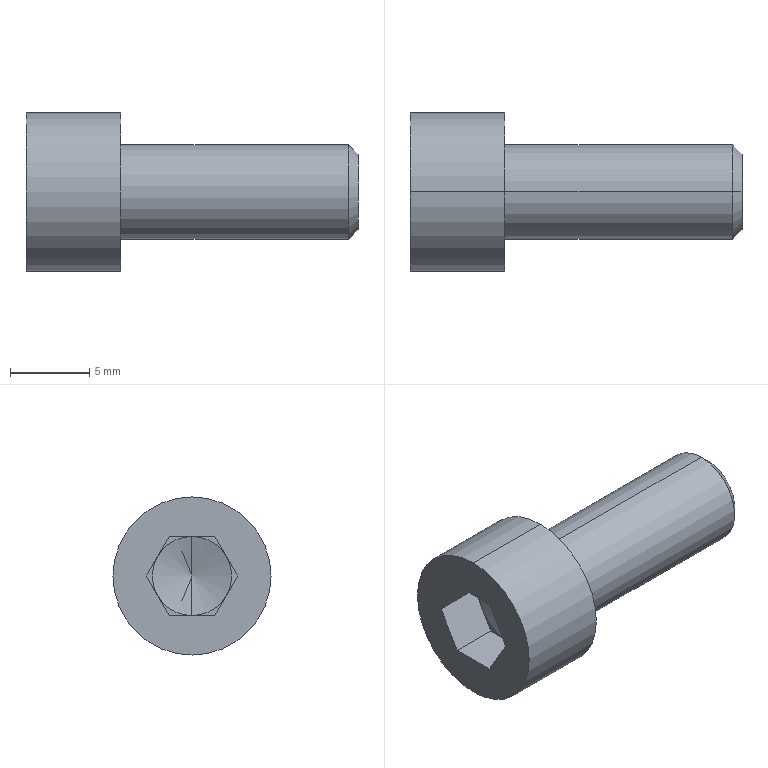Part | STEP file | 0232_301_CBM6-15 | 1 solid | 23 faces | box 21 x 10 x 10 mm | volume 822.712 mm3 | plane 15 | cylinder 4 | cone 4 | commonest cylinder face diameters 6 x2 10 x2
STEP:
#1=CARTESIAN_POINT('',(0.,0.,0.));
#2=DIRECTION('',(0.,0.,1.));
#3=DIRECTION('',(1.,0.,0.));
#4=AXIS2_PLACEMENT_3D('',#1,#2,#3);
#5=CARTESIAN_POINT('',(0.,0.,-3.));
#6=VERTEX_POINT('',#5);
#7=CARTESIAN_POINT('',(0.,0.,3.));
#8=VERTEX_POINT('',#7);
#9=CARTESIAN_POINT('',(0.,0.,0.));
#10=DIRECTION('',(1.,0.,0.));
#11=DIRECTION('',(0.,0.,-1.));
#12=AXIS2_PLACEMENT_3D('',#9,#10,#11);
#13=CIRCLE('',#12,3.);
#14=CARTESIAN_POINT('',(7.193,0.,0.));
#15=DIRECTION('',(1.,0.,0.));
#16=DIRECTION('',(0.,0.,-1.));
#17=AXIS2_PLACEMENT_3D('',#14,#15,#16);
#18=CYLINDRICAL_SURFACE('',#17,3.);
#19=CARTESIAN_POINT('',(0.,-7.193));
#20=DIRECTION('',(1.,0.));
#21=VECTOR('',#20,1.);
#22=LINE('',#19,#21);
#23=(GEOMETRIC_REPRESENTATION_CONTEXT(2)PARAMETRIC_REPRESENTATION_CONTEXT()REPRESENTATION_CONTEXT('',''));
#24=DEFINITIONAL_REPRESENTATION('',(#22),#23);
#25=PCURVE('',#18,#24);
#26=CARTESIAN_POINT('',(0.,4.,0.));
#27=DIRECTION('',(1.,0.,0.));
#28=DIRECTION('',(0.,0.,-1.));
#29=AXIS2_PLACEMENT_3D('',#26,#27,#28);
#30=PLANE('',#29);
#31=CARTESIAN_POINT('',(0.,-4.));
#32=DIRECTION('',(1.,0.));
#33=AXIS2_PLACEMENT_2D('',#31,#32);
#34=CIRCLE('',#33,3.);
#35=(GEOMETRIC_REPRESENTATION_CONTEXT(2)PARAMETRIC_REPRESENTATION_CONTEXT()REPRESENTATION_CONTEXT('',''));
#36=DEFINITIONAL_REPRESENTATION('',(#34),#35);
#37=PCURVE('',#30,#36);
#38=SURFACE_CURVE('',#13,(#25,#37),.PCURVE_S1.);
#39=EDGE_CURVE('',#6,#8,#38,.T.);
#40=ORIENTED_EDGE('',*,*,#39,.T.);
#41=CARTESIAN_POINT('',(14.386,0.,3.));
#42=VERTEX_POINT('',#41);
#43=CARTESIAN_POINT('',(7.193,0.,3.));
#44=DIRECTION('',(1.,0.,0.));
#45=VECTOR('',#44,1.);
#46=LINE('',#43,#45);
#47=CARTESIAN_POINT('',(3.142,0.));
#48=DIRECTION('',(0.,1.));
#49=VECTOR('',#48,1.);
#50=LINE('',#47,#49);
#51=(GEOMETRIC_REPRESENTATION_CONTEXT(2)PARAMETRIC_REPRESENTATION_CONTEXT()REPRESENTATION_CONTEXT('',''));
#52=DEFINITIONAL_REPRESENTATION('',(#50),#51);
#53=PCURVE('',#18,#52);
#54=CARTESIAN_POINT('',(7.193,0.,0.));
#55=DIRECTION('',(1.,0.,0.));
#56=DIRECTION('',(0.,0.,-1.));
#57=AXIS2_PLACEMENT_3D('',#54,#55,#56);
#58=CYLINDRICAL_SURFACE('',#57,3.);
#59=CARTESIAN_POINT('',(3.142,0.));
#60=DIRECTION('',(0.,1.));
#61=VECTOR('',#60,1.);
#62=LINE('',#59,#61);
#63=(GEOMETRIC_REPRESENTATION_CONTEXT(2)PARAMETRIC_REPRESENTATION_CONTEXT()REPRESENTATION_CONTEXT('',''));
#64=DEFINITIONAL_REPRESENTATION('',(#62),#63);
#65=PCURVE('',#58,#64);
#66=SURFACE_CURVE('',#46,(#53,#65),.PCURVE_S1.);
#67=EDGE_CURVE('',#8,#42,#66,.T.);
#68=ORIENTED_EDGE('',*,*,#67,.T.);
#69=CARTESIAN_POINT('',(14.386,0.,-3.));
#70=VERTEX_POINT('',#69);
#71=CARTESIAN_POINT('',(14.386,0.,0.));
#72=DIRECTION('',(-1.,0.,0.));
#73=DIRECTION('',(0.,0.,-1.));
#74=AXIS2_PLACEMENT_3D('',#71,#72,#73);
#75=CIRCLE('',#74,3.);
#76=CARTESIAN_POINT('',(6.283,7.193));
#77=DIRECTION('',(-1.,0.));
#78=VECTOR('',#77,1.);
#79=LINE('',#76,#78);
#80=(GEOMETRIC_REPRESENTATION_CONTEXT(2)PARAMETRIC_REPRESENTATION_CONTEXT()REPRESENTATION_CONTEXT('',''));
#81=DEFINITIONAL_REPRESENTATION('',(#79),#80);
#82=PCURVE('',#18,#81);
#83=CARTESIAN_POINT('',(14.387,0.,0.));
#84=DIRECTION('',(-1.,0.,0.));
#85=DIRECTION('',(0.,0.,1.));
#86=AXIS2_PLACEMENT_3D('',#83,#84,#85);
#87=CONICAL_SURFACE('',#86,3.,0.7854);
#88=CARTESIAN_POINT('',(-3.142,0.));
#89=DIRECTION('',(1.,0.));
#90=VECTOR('',#89,1.);
#91=LINE('',#88,#90);
#92=(GEOMETRIC_REPRESENTATION_CONTEXT(2)PARAMETRIC_REPRESENTATION_CONTEXT()REPRESENTATION_CONTEXT('',''));
#93=DEFINITIONAL_REPRESENTATION('',(#91),#92);
#94=PCURVE('',#87,#93);
#95=SURFACE_CURVE('',#75,(#82,#94),.PCURVE_S1.);
#96=EDGE_CURVE('',#42,#70,#95,.T.);
#97=ORIENTED_EDGE('',*,*,#96,.T.);
#98=CARTESIAN_POINT('',(7.193,0.,-3.));
#99=DIRECTION('',(1.,0.,0.));
#100=VECTOR('',#99,1.);
#101=LINE('',#98,#100);
#102=CARTESIAN_POINT('',(0.,0.));
#103=DIRECTION('',(0.,1.));
#104=VECTOR('',#103,1.);
#105=LINE('',#102,#104);
#106=(GEOMETRIC_REPRESENTATION_CONTEXT(2)PARAMETRIC_REPRESENTATION_CONTEXT()REPRESENTATION_CONTEXT('',''));
#107=DEFINITIONAL_REPRESENTATION('',(#105),#106);
#108=PCURVE('',#18,#107);
#109=CARTESIAN_POINT('',(6.283,0.));
#110=DIRECTION('',(0.,1.));
#111=VECTOR('',#110,1.);
#112=LINE('',#109,#111);
#113=(GEOMETRIC_REPRESENTATION_CONTEXT(2)PARAMETRIC_REPRESENTATION_CONTEXT()REPRESENTATION_CONTEXT('',''));
#114=DEFINITIONAL_REPRESENTATION('',(#112),#113);
#115=PCURVE('',#58,#114);
#116=SURFACE_CURVE('',#101,(#108,#115),.PCURVE_S1.);
#117=EDGE_CURVE('',#6,#70,#116,.T.);
#118=ORIENTED_EDGE('',*,*,#117,.F.);
#119=EDGE_LOOP('',(#40,#68,#97,#118));
#120=FACE_BOUND('',#119,.T.);
#121=ADVANCED_FACE('',(#120),#18,.T.);
#122=CARTESIAN_POINT('',(15.,0.,2.386));
#123=VERTEX_POINT('',#122);
#124=CARTESIAN_POINT('',(15.,0.,-2.386));
#125=VERTEX_POINT('',#124);
#126=CARTESIAN_POINT('',(15.,0.,0.));
#127=DIRECTION('',(-1.,0.,0.));
#128=DIRECTION('',(0.,0.,1.));
#129=AXIS2_PLACEMENT_3D('',#126,#127,#128);
#130=CIRCLE('',#129,2.386);
#131=CARTESIAN_POINT('',(0.,-0.6135));
#132=DIRECTION('',(1.,0.));
#133=VECTOR('',#132,1.);
#134=LINE('',#131,#133);
#135=(GEOMETRIC_REPRESENTATION_CONTEXT(2)PARAMETRIC_REPRESENTATION_CONTEXT()REPRESENTATION_CONTEXT('',''));
#136=DEFINITIONAL_REPRESENTATION('',(#134),#135);
#137=PCURVE('',#87,#136);
#138=CARTESIAN_POINT('',(15.,1.193,0.));
#139=DIRECTION('',(1.,0.,0.));
#140=DIRECTION('',(0.,0.,-1.));
#141=AXIS2_PLACEMENT_3D('',#138,#139,#140);
#142=PLANE('',#141);
#143=CARTESIAN_POINT('',(-2.386,-1.193));
#144=CARTESIAN_POINT('',(-2.386,2.94));
#145=CARTESIAN_POINT('',(1.193,0.8735));
#146=CARTESIAN_POINT('',(4.773,-1.193));
#147=CARTESIAN_POINT('',(1.193,-3.26));
#148=CARTESIAN_POINT('',(-2.386,-5.327));
#149=CARTESIAN_POINT('',(-2.386,-1.193));
#150=(BOUNDED_CURVE()B_SPLINE_CURVE(2,(#143,#144,#145,#146,#147,#148,#149),.UNSPECIFIED.,.T.,.F.)B_SPLINE_CURVE_WITH_KNOTS((1,2,2,2,2,1),(-2.094,0.,2.094,4.189,6.283,8.378),.UNSPECIFIED.)CURVE()GEOMETRIC_REPRESENTATION_ITEM()RATIONAL_B_SPLINE_CURVE((1.,0.5,1.,0.5,1.,0.5,1.))REPRESENTATION_ITEM(''));
#151=(GEOMETRIC_REPRESENTATION_CONTEXT(2)PARAMETRIC_REPRESENTATION_CONTEXT()REPRESENTATION_CONTEXT('',''));
#152=DEFINITIONAL_REPRESENTATION('',(#150),#151);
#153=PCURVE('',#142,#152);
#154=SURFACE_CURVE('',#130,(#137,#153),.PCURVE_S1.);
#155=EDGE_CURVE('',#123,#125,#154,.T.);
#156=ORIENTED_EDGE('',*,*,#155,.T.);
#157=CARTESIAN_POINT('',(14.387,0.,-3.));
#158=DIRECTION('',(-0.7071,0.,-0.7071));
#159=VECTOR('',#158,1.);
#160=LINE('',#157,#159);
#161=CARTESIAN_POINT('',(3.142,0.));
#162=DIRECTION('',(0.,1.));
#163=VECTOR('',#162,1.);
#164=LINE('',#161,#163);
#165=(GEOMETRIC_REPRESENTATION_CONTEXT(2)PARAMETRIC_REPRESENTATION_CONTEXT()REPRESENTATION_CONTEXT('',''));
#166=DEFINITIONAL_REPRESENTATION('',(#164),#165);
#167=PCURVE('',#87,#166);
#168=CARTESIAN_POINT('',(14.387,0.,0.));
#169=DIRECTION('',(-1.,0.,0.));
#170=DIRECTION('',(0.,0.,1.));
#171=AXIS2_PLACEMENT_3D('',#168,#169,#170);
#172=CONICAL_SURFACE('',#171,3.,0.7854);
#173=CARTESIAN_POINT('',(3.142,0.));
#174=DIRECTION('',(0.,1.));
#175=VECTOR('',#174,1.);
#176=LINE('',#173,#175);
#177=(GEOMETRIC_REPRESENTATION_CONTEXT(2)PARAMETRIC_REPRESENTATION_CONTEXT()REPRESENTATION_CONTEXT('',''));
#178=DEFINITIONAL_REPRESENTATION('',(#176),#177);
#179=PCURVE('',#172,#178);
#180=SURFACE_CURVE('',#160,(#167,#179),.PCURVE_S1.);
#181=EDGE_CURVE('',#125,#70,#180,.T.);
#182=ORIENTED_EDGE('',*,*,#181,.T.);
#183=ORIENTED_EDGE('',*,*,#96,.F.);
#184=CARTESIAN_POINT('',(14.387,0.,3.));
#185=DIRECTION('',(-0.7071,0.,0.7071));
#186=VECTOR('',#185,1.);
#187=LINE('',#184,#186);
#188=CARTESIAN_POINT('',(0.,0.));
#189=DIRECTION('',(0.,1.));
#190=VECTOR('',#189,1.);
#191=LINE('',#188,#190);
#192=(GEOMETRIC_REPRESENTATION_CONTEXT(2)PARAMETRIC_REPRESENTATION_CONTEXT()REPRESENTATION_CONTEXT('',''));
#193=DEFINITIONAL_REPRESENTATION('',(#191),#192);
#194=PCURVE('',#87,#193);
#195=CARTESIAN_POINT('',(6.283,0.));
#196=DIRECTION('',(0.,1.));
#197=VECTOR('',#196,1.);
#198=LINE('',#195,#197);
#199=(GEOMETRIC_REPRESENTATION_CONTEXT(2)PARAMETRIC_REPRESENTATION_CONTEXT()REPRESENTATION_CONTEXT('',''));
#200=DEFINITIONAL_REPRESENTATION('',(#198),#199);
#201=PCURVE('',#172,#200);
#202=SURFACE_CURVE('',#187,(#194,#201),.PCURVE_S1.);
#203=EDGE_CURVE('',#123,#42,#202,.T.);
#204=ORIENTED_EDGE('',*,*,#203,.F.);
#205=EDGE_LOOP('',(#156,#182,#183,#204));
#206=FACE_BOUND('',#205,.T.);
#207=ADVANCED_FACE('',(#206),#87,.T.);
#208=CARTESIAN_POINT('',(-6.,0.,-5.));
#209=VERTEX_POINT('',#208);
#210=CARTESIAN_POINT('',(-6.,0.,5.));
#211=VERTEX_POINT('',#210);
#212=CARTESIAN_POINT('',(-6.,0.,0.));
#213=DIRECTION('',(1.,0.,0.));
#214=DIRECTION('',(0.,0.,-1.));
#215=AXIS2_PLACEMENT_3D('',#212,#213,#214);
#216=CIRCLE('',#215,5.);
#217=CARTESIAN_POINT('',(-3.,0.,0.));
#218=DIRECTION('',(1.,0.,0.));
#219=DIRECTION('',(0.,0.,-1.));
#220=AXIS2_PLACEMENT_3D('',#217,#218,#219);
#221=CYLINDRICAL_SURFACE('',#220,5.);
#222=CARTESIAN_POINT('',(0.,-3.));
#223=DIRECTION('',(1.,0.));
#224=VECTOR('',#223,1.);
#225=LINE('',#222,#224);
#226=(GEOMETRIC_REPRESENTATION_CONTEXT(2)PARAMETRIC_REPRESENTATION_CONTEXT()REPRESENTATION_CONTEXT('',''));
#227=DEFINITIONAL_REPRESENTATION('',(#225),#226);
#228=PCURVE('',#221,#227);
#229=CARTESIAN_POINT('',(-6.,2.5,0.));
#230=DIRECTION('',(-1.,0.,0.));
#231=DIRECTION('',(0.,0.,1.));
#232=AXIS2_PLACEMENT_3D('',#229,#230,#231);
#233=PLANE('',#232);
#234=CARTESIAN_POINT('',(-5.,-2.5));
#235=CARTESIAN_POINT('',(-5.,6.16));
#236=CARTESIAN_POINT('',(2.5,1.83));
#237=CARTESIAN_POINT('',(10.,-2.5));
#238=CARTESIAN_POINT('',(2.5,-6.83));
#239=CARTESIAN_POINT('',(-5.,-11.16));
#240=CARTESIAN_POINT('',(-5.,-2.5));
#241=(BOUNDED_CURVE()B_SPLINE_CURVE(2,(#234,#235,#236,#237,#238,#239,#240),.UNSPECIFIED.,.T.,.F.)B_SPLINE_CURVE_WITH_KNOTS((1,2,2,2,2,1),(-2.094,0.,2.094,4.189,6.283,8.378),.UNSPECIFIED.)CURVE()GEOMETRIC_REPRESENTATION_ITEM()RATIONAL_B_SPLINE_CURVE((1.,0.5,1.,0.5,1.,0.5,1.))REPRESENTATION_ITEM(''));
#242=(GEOMETRIC_REPRESENTATION_CONTEXT(2)PARAMETRIC_REPRESENTATION_CONTEXT()REPRESENTATION_CONTEXT('',''));
#243=DEFINITIONAL_REPRESENTATION('',(#241),#242);
#244=PCURVE('',#233,#243);
#245=SURFACE_CURVE('',#216,(#228,#244),.PCURVE_S1.);
#246=EDGE_CURVE('',#209,#211,#245,.T.);
#247=ORIENTED_EDGE('',*,*,#246,.T.);
#248=CARTESIAN_POINT('',(0.,0.,5.));
#249=VERTEX_POINT('',#248);
#250=CARTESIAN_POINT('',(-3.,0.,5.));
#251=DIRECTION('',(1.,0.,0.));
#252=VECTOR('',#251,1.);
#253=LINE('',#250,#252);
#254=CARTESIAN_POINT('',(3.142,0.));
#255=DIRECTION('',(0.,1.));
#256=VECTOR('',#255,1.);
#257=LINE('',#254,#256);
#258=(GEOMETRIC_REPRESENTATION_CONTEXT(2)PARAMETRIC_REPRESENTATION_CONTEXT()REPRESENTATION_CONTEXT('',''));
#259=DEFINITIONAL_REPRESENTATION('',(#257),#258);
#260=PCURVE('',#221,#259);
#261=CARTESIAN_POINT('',(-3.,0.,0.));
#262=DIRECTION('',(1.,0.,0.));
#263=DIRECTION('',(0.,0.,-1.));
#264=AXIS2_PLACEMENT_3D('',#261,#262,#263);
#265=CYLINDRICAL_SURFACE('',#264,5.);
#266=CARTESIAN_POINT('',(3.142,0.));
#267=DIRECTION('',(0.,1.));
#268=VECTOR('',#267,1.);
#269=LINE('',#266,#268);
#270=(GEOMETRIC_REPRESENTATION_CONTEXT(2)PARAMETRIC_REPRESENTATION_CONTEXT()REPRESENTATION_CONTEXT('',''));
#271=DEFINITIONAL_REPRESENTATION('',(#269),#270);
#272=PCURVE('',#265,#271);
#273=SURFACE_CURVE('',#253,(#260,#272),.PCURVE_S1.);
#274=EDGE_CURVE('',#211,#249,#273,.T.);
#275=ORIENTED_EDGE('',*,*,#274,.T.);
#276=CARTESIAN_POINT('',(0.,0.,-5.));
#277=VERTEX_POINT('',#276);
#278=CARTESIAN_POINT('',(0.,0.,0.));
#279=DIRECTION('',(1.,0.,0.));
#280=DIRECTION('',(0.,0.,-1.));
#281=AXIS2_PLACEMENT_3D('',#278,#279,#280);
#282=CIRCLE('',#281,5.);
#283=CARTESIAN_POINT('',(0.,3.));
#284=DIRECTION('',(1.,0.));
#285=VECTOR('',#284,1.);
#286=LINE('',#283,#285);
#287=(GEOMETRIC_REPRESENTATION_CONTEXT(2)PARAMETRIC_REPRESENTATION_CONTEXT()REPRESENTATION_CONTEXT('',''));
#288=DEFINITIONAL_REPRESENTATION('',(#286),#287);
#289=PCURVE('',#221,#288);
#290=CARTESIAN_POINT('',(0.,-4.));
#291=DIRECTION('',(1.,0.));
#292=AXIS2_PLACEMENT_2D('',#290,#291);
#293=CIRCLE('',#292,5.);
#294=(GEOMETRIC_REPRESENTATION_CONTEXT(2)PARAMETRIC_REPRESENTATION_CONTEXT()REPRESENTATION_CONTEXT('',''));
#295=DEFINITIONAL_REPRESENTATION('',(#293),#294);
#296=PCURVE('',#30,#295);
#297=SURFACE_CURVE('',#282,(#289,#296),.PCURVE_S1.);
#298=EDGE_CURVE('',#277,#249,#297,.T.);
#299=ORIENTED_EDGE('',*,*,#298,.F.);
#300=CARTESIAN_POINT('',(-3.,0.,-5.));
#301=DIRECTION('',(1.,0.,0.));
#302=VECTOR('',#301,1.);
#303=LINE('',#300,#302);
#304=CARTESIAN_POINT('',(0.,0.));
#305=DIRECTION('',(0.,1.));
#306=VECTOR('',#305,1.);
#307=LINE('',#304,#306);
#308=(GEOMETRIC_REPRESENTATION_CONTEXT(2)PARAMETRIC_REPRESENTATION_CONTEXT()REPRESENTATION_CONTEXT('',''));
#309=DEFINITIONAL_REPRESENTATION('',(#307),#308);
#310=PCURVE('',#221,#309);
#311=CARTESIAN_POINT('',(6.283,0.));
#312=DIRECTION('',(0.,1.));
#313=VECTOR('',#312,1.);
#314=LINE('',#311,#313);
#315=(GEOMETRIC_REPRESENTATION_CONTEXT(2)PARAMETRIC_REPRESENTATION_CONTEXT()REPRESENTATION_CONTEXT('',''));
#316=DEFINITIONAL_REPRESENTATION('',(#314),#315);
#317=PCURVE('',#265,#316);
#318=SURFACE_CURVE('',#303,(#310,#317),.PCURVE_S1.);
#319=EDGE_CURVE('',#209,#277,#318,.T.);
#320=ORIENTED_EDGE('',*,*,#319,.F.);
#321=EDGE_LOOP('',(#247,#275,#299,#320));
#322=FACE_BOUND('',#321,.T.);
#323=ADVANCED_FACE('',(#322),#221,.T.);
#324=CARTESIAN_POINT('',(-3.,-2.165,1.25));
#325=VERTEX_POINT('',#324);
#326=CARTESIAN_POINT('',(-3.,0.,2.5));
#327=VERTEX_POINT('',#326);
#328=CARTESIAN_POINT('',(-3.,0.,0.));
#329=DIRECTION('',(-1.,0.,0.));
#330=DIRECTION('',(0.,0.,1.));
#331=AXIS2_PLACEMENT_3D('',#328,#329,#330);
#332=CIRCLE('',#331,2.5);
#333=CARTESIAN_POINT('',(-3.,0.,0.));
#334=DIRECTION('',(-1.,0.,0.));
#335=DIRECTION('',(0.,0.,1.));
#336=AXIS2_PLACEMENT_3D('',#333,#334,#335);
#337=CONICAL_SURFACE('',#336,2.5,1.309);
#338=CARTESIAN_POINT('',(0.,0.));
#339=DIRECTION('',(1.,0.));
#340=VECTOR('',#339,1.);
#341=LINE('',#338,#340);
#342=(GEOMETRIC_REPRESENTATION_CONTEXT(2)PARAMETRIC_REPRESENTATION_CONTEXT()REPRESENTATION_CONTEXT('',''));
#343=DEFINITIONAL_REPRESENTATION('',(#341),#342);
#344=PCURVE('',#337,#343);
#345=CARTESIAN_POINT('',(-3.,0.,0.));
#346=DIRECTION('',(1.,0.,0.));
#347=DIRECTION('',(0.,0.,-1.));
#348=AXIS2_PLACEMENT_3D('',#345,#346,#347);
#349=PLANE('',#348);
#350=CARTESIAN_POINT('',(-2.5,0.));
#351=CARTESIAN_POINT('',(-2.5,4.33));
#352=CARTESIAN_POINT('',(1.25,2.165));
#353=CARTESIAN_POINT('',(5.,0.));
#354=CARTESIAN_POINT('',(1.25,-2.165));
#355=CARTESIAN_POINT('',(-2.5,-4.33));
#356=CARTESIAN_POINT('',(-2.5,0.));
#357=(BOUNDED_CURVE()B_SPLINE_CURVE(2,(#350,#351,#352,#353,#354,#355,#356),.UNSPECIFIED.,.T.,.F.)B_SPLINE_CURVE_WITH_KNOTS((1,2,2,2,2,1),(-2.094,0.,2.094,4.189,6.283,8.378),.UNSPECIFIED.)CURVE()GEOMETRIC_REPRESENTATION_ITEM()RATIONAL_B_SPLINE_CURVE((1.,0.5,1.,0.5,1.,0.5,1.))REPRESENTATION_ITEM(''));
#358=(GEOMETRIC_REPRESENTATION_CONTEXT(2)PARAMETRIC_REPRESENTATION_CONTEXT()REPRESENTATION_CONTEXT('',''));
#359=DEFINITIONAL_REPRESENTATION('',(#357),#358);
#360=PCURVE('',#349,#359);
#361=SURFACE_CURVE('',#332,(#344,#360),.PCURVE_S1.);
#362=EDGE_CURVE('',#325,#327,#361,.T.);
#363=ORIENTED_EDGE('',*,*,#362,.F.);
#364=CARTESIAN_POINT('',(-3.,-2.165,-1.25));
#365=VERTEX_POINT('',#364);
#366=CARTESIAN_POINT('',(-3.,0.,0.));
#367=DIRECTION('',(1.,0.,0.));
#368=DIRECTION('',(0.,0.,1.));
#369=AXIS2_PLACEMENT_3D('',#366,#367,#368);
#370=CIRCLE('',#369,2.5);
#371=CARTESIAN_POINT('',(6.283,0.));
#372=DIRECTION('',(-1.,0.));
#373=VECTOR('',#372,1.);
#374=LINE('',#371,#373);
#375=(GEOMETRIC_REPRESENTATION_CONTEXT(2)PARAMETRIC_REPRESENTATION_CONTEXT()REPRESENTATION_CONTEXT('',''));
#376=DEFINITIONAL_REPRESENTATION('',(#374),#375);
#377=PCURVE('',#337,#376);
#378=CARTESIAN_POINT('',(-3.,0.,0.));
#379=DIRECTION('',(1.,0.,0.));
#380=DIRECTION('',(0.,0.,-1.));
#381=AXIS2_PLACEMENT_3D('',#378,#379,#380);
#382=PLANE('',#381);
#383=CARTESIAN_POINT('',(0.,0.));
#384=DIRECTION('',(-1.,0.));
#385=AXIS2_PLACEMENT_2D('',#383,#384);
#386=CIRCLE('',#385,2.5);
#387=(GEOMETRIC_REPRESENTATION_CONTEXT(2)PARAMETRIC_REPRESENTATION_CONTEXT()REPRESENTATION_CONTEXT('',''));
#388=DEFINITIONAL_REPRESENTATION('',(#386),#387);
#389=PCURVE('',#382,#388);
#390=SURFACE_CURVE('',#370,(#377,#389),.PCURVE_S1.);
#391=EDGE_CURVE('',#325,#365,#390,.T.);
#392=ORIENTED_EDGE('',*,*,#391,.T.);
#393=CARTESIAN_POINT('',(-3.,0.,-2.5));
#394=VERTEX_POINT('',#393);
#395=CARTESIAN_POINT('',(-3.,0.,0.));
#396=DIRECTION('',(1.,0.,0.));
#397=DIRECTION('',(0.,0.,1.));
#398=AXIS2_PLACEMENT_3D('',#395,#396,#397);
#399=CIRCLE('',#398,2.5);
#400=CARTESIAN_POINT('',(6.283,0.));
#401=DIRECTION('',(-1.,0.));
#402=VECTOR('',#401,1.);
#403=LINE('',#400,#402);
#404=(GEOMETRIC_REPRESENTATION_CONTEXT(2)PARAMETRIC_REPRESENTATION_CONTEXT()REPRESENTATION_CONTEXT('',''));
#405=DEFINITIONAL_REPRESENTATION('',(#403),#404);
#406=PCURVE('',#337,#405);
#407=CARTESIAN_POINT('',(-3.,0.,0.));
#408=DIRECTION('',(1.,0.,0.));
#409=DIRECTION('',(0.,0.,-1.));
#410=AXIS2_PLACEMENT_3D('',#407,#408,#409);
#411=PLANE('',#410);
#412=CARTESIAN_POINT('',(0.,0.));
#413=DIRECTION('',(-1.,0.));
#414=AXIS2_PLACEMENT_2D('',#412,#413);
#415=CIRCLE('',#414,2.5);
#416=(GEOMETRIC_REPRESENTATION_CONTEXT(2)PARAMETRIC_REPRESENTATION_CONTEXT()REPRESENTATION_CONTEXT('',''));
#417=DEFINITIONAL_REPRESENTATION('',(#415),#416);
#418=PCURVE('',#411,#417);
#419=SURFACE_CURVE('',#399,(#406,#418),.PCURVE_S1.);
#420=EDGE_CURVE('',#365,#394,#419,.T.);
#421=ORIENTED_EDGE('',*,*,#420,.T.);
#422=CARTESIAN_POINT('',(-2.33,0.,0.));
#423=VERTEX_POINT('',#422);
#424=CARTESIAN_POINT('',(-3.,0.,-2.5));
#425=DIRECTION('',(-0.2588,0.,-0.9659));
#426=VECTOR('',#425,1.);
#427=LINE('',#424,#426);
#428=CARTESIAN_POINT('',(3.142,0.));
#429=DIRECTION('',(0.,1.));
#430=VECTOR('',#429,1.);
#431=LINE('',#428,#430);
#432=(GEOMETRIC_REPRESENTATION_CONTEXT(2)PARAMETRIC_REPRESENTATION_CONTEXT()REPRESENTATION_CONTEXT('',''));
#433=DEFINITIONAL_REPRESENTATION('',(#431),#432);
#434=PCURVE('',#337,#433);
#435=CARTESIAN_POINT('',(-3.,0.,0.));
#436=DIRECTION('',(-1.,0.,0.));
#437=DIRECTION('',(0.,0.,1.));
#438=AXIS2_PLACEMENT_3D('',#435,#436,#437);
#439=CONICAL_SURFACE('',#438,2.5,1.309);
#440=CARTESIAN_POINT('',(3.142,0.));
#441=DIRECTION('',(0.,1.));
#442=VECTOR('',#441,1.);
#443=LINE('',#440,#442);
#444=(GEOMETRIC_REPRESENTATION_CONTEXT(2)PARAMETRIC_REPRESENTATION_CONTEXT()REPRESENTATION_CONTEXT('',''));
#445=DEFINITIONAL_REPRESENTATION('',(#443),#444);
#446=PCURVE('',#439,#445);
#447=SURFACE_CURVE('',#427,(#434,#446),.PCURVE_S1.);
#448=EDGE_CURVE('',#423,#394,#447,.T.);
#449=ORIENTED_EDGE('',*,*,#448,.F.);
#450=CARTESIAN_POINT('',(-3.,0.,2.5));
#451=DIRECTION('',(-0.2588,0.,0.9659));
#452=VECTOR('',#451,1.);
#453=LINE('',#450,#452);
#454=CARTESIAN_POINT('',(6.283,0.));
#455=DIRECTION('',(0.,1.));
#456=VECTOR('',#455,1.);
#457=LINE('',#454,#456);
#458=(GEOMETRIC_REPRESENTATION_CONTEXT(2)PARAMETRIC_REPRESENTATION_CONTEXT()REPRESENTATION_CONTEXT('',''));
#459=DEFINITIONAL_REPRESENTATION('',(#457),#458);
#460=PCURVE('',#337,#459);
#461=CARTESIAN_POINT('',(0.,0.));
#462=DIRECTION('',(0.,1.));
#463=VECTOR('',#462,1.);
#464=LINE('',#461,#463);
#465=(GEOMETRIC_REPRESENTATION_CONTEXT(2)PARAMETRIC_REPRESENTATION_CONTEXT()REPRESENTATION_CONTEXT('',''));
#466=DEFINITIONAL_REPRESENTATION('',(#464),#465);
#467=PCURVE('',#439,#466);
#468=SURFACE_CURVE('',#453,(#460,#467),.PCURVE_S1.);
#469=EDGE_CURVE('',#423,#327,#468,.T.);
#470=ORIENTED_EDGE('',*,*,#469,.T.);
#471=EDGE_LOOP('',(#363,#392,#421,#449,#470));
#472=FACE_BOUND('',#471,.F.);
#473=ADVANCED_FACE('',(#472),#337,.F.);
#474=ORIENTED_EDGE('',*,*,#67,.F.);
#475=CARTESIAN_POINT('',(0.,0.,0.));
#476=DIRECTION('',(1.,0.,0.));
#477=DIRECTION('',(0.,0.,-1.));
#478=AXIS2_PLACEMENT_3D('',#475,#476,#477);
#479=CIRCLE('',#478,3.);
#480=CARTESIAN_POINT('',(0.,-7.193));
#481=DIRECTION('',(1.,0.));
#482=VECTOR('',#481,1.);
#483=LINE('',#480,#482);
#484=(GEOMETRIC_REPRESENTATION_CONTEXT(2)PARAMETRIC_REPRESENTATION_CONTEXT()REPRESENTATION_CONTEXT('',''));
#485=DEFINITIONAL_REPRESENTATION('',(#483),#484);
#486=PCURVE('',#58,#485);
#487=CARTESIAN_POINT('',(0.,-4.));
#488=DIRECTION('',(1.,0.));
#489=AXIS2_PLACEMENT_2D('',#487,#488);
#490=CIRCLE('',#489,3.);
#491=(GEOMETRIC_REPRESENTATION_CONTEXT(2)PARAMETRIC_REPRESENTATION_CONTEXT()REPRESENTATION_CONTEXT('',''));
#492=DEFINITIONAL_REPRESENTATION('',(#490),#491);
#493=PCURVE('',#30,#492);
#494=SURFACE_CURVE('',#479,(#486,#493),.PCURVE_S1.);
#495=EDGE_CURVE('',#8,#6,#494,.T.);
#496=ORIENTED_EDGE('',*,*,#495,.T.);
#497=ORIENTED_EDGE('',*,*,#117,.T.);
#498=CARTESIAN_POINT('',(14.386,0.,0.));
#499=DIRECTION('',(-1.,0.,0.));
#500=DIRECTION('',(0.,0.,-1.));
#501=AXIS2_PLACEMENT_3D('',#498,#499,#500);
#502=CIRCLE('',#501,3.);
#503=CARTESIAN_POINT('',(6.283,7.193));
#504=DIRECTION('',(-1.,0.));
#505=VECTOR('',#504,1.);
#506=LINE('',#503,#505);
#507=(GEOMETRIC_REPRESENTATION_CONTEXT(2)PARAMETRIC_REPRESENTATION_CONTEXT()REPRESENTATION_CONTEXT('',''));
#508=DEFINITIONAL_REPRESENTATION('',(#506),#507);
#509=PCURVE('',#58,#508);
#510=CARTESIAN_POINT('',(3.142,0.));
#511=DIRECTION('',(1.,0.));
#512=VECTOR('',#511,1.);
#513=LINE('',#510,#512);
#514=(GEOMETRIC_REPRESENTATION_CONTEXT(2)PARAMETRIC_REPRESENTATION_CONTEXT()REPRESENTATION_CONTEXT('',''));
#515=DEFINITIONAL_REPRESENTATION('',(#513),#514);
#516=PCURVE('',#172,#515);
#517=SURFACE_CURVE('',#502,(#509,#516),.PCURVE_S1.);
#518=EDGE_CURVE('',#70,#42,#517,.T.);
#519=ORIENTED_EDGE('',*,*,#518,.T.);
#520=EDGE_LOOP('',(#474,#496,#497,#519));
#521=FACE_BOUND('',#520,.T.);
#522=ADVANCED_FACE('',(#521),#58,.T.);
#523=ORIENTED_EDGE('',*,*,#39,.F.);
#524=ORIENTED_EDGE('',*,*,#495,.F.);
#525=EDGE_LOOP('',(#523,#524));
#526=FACE_BOUND('',#525,.T.);
#527=ORIENTED_EDGE('',*,*,#298,.T.);
#528=CARTESIAN_POINT('',(0.,0.,0.));
#529=DIRECTION('',(1.,0.,0.));
#530=DIRECTION('',(0.,0.,-1.));
#531=AXIS2_PLACEMENT_3D('',#528,#529,#530);
#532=CIRCLE('',#531,5.);
#533=CARTESIAN_POINT('',(0.,-4.));
#534=DIRECTION('',(1.,0.));
#535=AXIS2_PLACEMENT_2D('',#533,#534);
#536=CIRCLE('',#535,5.);
#537=(GEOMETRIC_REPRESENTATION_CONTEXT(2)PARAMETRIC_REPRESENTATION_CONTEXT()REPRESENTATION_CONTEXT('',''));
#538=DEFINITIONAL_REPRESENTATION('',(#536),#537);
#539=PCURVE('',#30,#538);
#540=CARTESIAN_POINT('',(0.,3.));
#541=DIRECTION('',(1.,0.));
#542=VECTOR('',#541,1.);
#543=LINE('',#540,#542);
#544=(GEOMETRIC_REPRESENTATION_CONTEXT(2)PARAMETRIC_REPRESENTATION_CONTEXT()REPRESENTATION_CONTEXT('',''));
#545=DEFINITIONAL_REPRESENTATION('',(#543),#544);
#546=PCURVE('',#265,#545);
#547=SURFACE_CURVE('',#532,(#539,#546),.PCURVE_S1.);
#548=EDGE_CURVE('',#249,#277,#547,.T.);
#549=ORIENTED_EDGE('',*,*,#548,.T.);
#550=EDGE_LOOP('',(#527,#549));
#551=FACE_BOUND('',#550,.T.);
#552=ADVANCED_FACE('',(#526,#551),#30,.T.);
#553=ORIENTED_EDGE('',*,*,#181,.F.);
#554=CARTESIAN_POINT('',(15.,0.,0.));
#555=DIRECTION('',(-1.,0.,0.));
#556=DIRECTION('',(0.,0.,1.));
#557=AXIS2_PLACEMENT_3D('',#554,#555,#556);
#558=CIRCLE('',#557,2.386);
#559=CARTESIAN_POINT('',(0.,-0.6135));
#560=DIRECTION('',(1.,0.));
#561=VECTOR('',#560,1.);
#562=LINE('',#559,#561);
#563=(GEOMETRIC_REPRESENTATION_CONTEXT(2)PARAMETRIC_REPRESENTATION_CONTEXT()REPRESENTATION_CONTEXT('',''));
#564=DEFINITIONAL_REPRESENTATION('',(#562),#563);
#565=PCURVE('',#172,#564);
#566=CARTESIAN_POINT('',(-2.386,-1.193));
#567=CARTESIAN_POINT('',(-2.386,2.94));
#568=CARTESIAN_POINT('',(1.193,0.8735));
#569=CARTESIAN_POINT('',(4.773,-1.193));
#570=CARTESIAN_POINT('',(1.193,-3.26));
#571=CARTESIAN_POINT('',(-2.386,-5.327));
#572=CARTESIAN_POINT('',(-2.386,-1.193));
#573=(BOUNDED_CURVE()B_SPLINE_CURVE(2,(#566,#567,#568,#569,#570,#571,#572),.UNSPECIFIED.,.T.,.F.)B_SPLINE_CURVE_WITH_KNOTS((1,2,2,2,2,1),(-2.094,0.,2.094,4.189,6.283,8.378),.UNSPECIFIED.)CURVE()GEOMETRIC_REPRESENTATION_ITEM()RATIONAL_B_SPLINE_CURVE((1.,0.5,1.,0.5,1.,0.5,1.))REPRESENTATION_ITEM(''));
#574=(GEOMETRIC_REPRESENTATION_CONTEXT(2)PARAMETRIC_REPRESENTATION_CONTEXT()REPRESENTATION_CONTEXT('',''));
#575=DEFINITIONAL_REPRESENTATION('',(#573),#574);
#576=PCURVE('',#142,#575);
#577=SURFACE_CURVE('',#558,(#565,#576),.PCURVE_S1.);
#578=EDGE_CURVE('',#125,#123,#577,.T.);
#579=ORIENTED_EDGE('',*,*,#578,.T.);
#580=ORIENTED_EDGE('',*,*,#203,.T.);
#581=ORIENTED_EDGE('',*,*,#518,.F.);
#582=EDGE_LOOP('',(#553,#579,#580,#581));
#583=FACE_BOUND('',#582,.T.);
#584=ADVANCED_FACE('',(#583),#172,.T.);
#585=ORIENTED_EDGE('',*,*,#274,.F.);
#586=CARTESIAN_POINT('',(-6.,0.,0.));
#587=DIRECTION('',(1.,0.,0.));
#588=DIRECTION('',(0.,0.,-1.));
#589=AXIS2_PLACEMENT_3D('',#586,#587,#588);
#590=CIRCLE('',#589,5.);
#591=CARTESIAN_POINT('',(0.,-3.));
#592=DIRECTION('',(1.,0.));
#593=VECTOR('',#592,1.);
#594=LINE('',#591,#593);
#595=(GEOMETRIC_REPRESENTATION_CONTEXT(2)PARAMETRIC_REPRESENTATION_CONTEXT()REPRESENTATION_CONTEXT('',''));
#596=DEFINITIONAL_REPRESENTATION('',(#594),#595);
#597=PCURVE('',#265,#596);
#598=CARTESIAN_POINT('',(-5.,-2.5));
#599=CARTESIAN_POINT('',(-5.,6.16));
#600=CARTESIAN_POINT('',(2.5,1.83));
#601=CARTESIAN_POINT('',(10.,-2.5));
#602=CARTESIAN_POINT('',(2.5,-6.83));
#603=CARTESIAN_POINT('',(-5.,-11.16));
#604=CARTESIAN_POINT('',(-5.,-2.5));
#605=(BOUNDED_CURVE()B_SPLINE_CURVE(2,(#598,#599,#600,#601,#602,#603,#604),.UNSPECIFIED.,.T.,.F.)B_SPLINE_CURVE_WITH_KNOTS((1,2,2,2,2,1),(-2.094,0.,2.094,4.189,6.283,8.378),.UNSPECIFIED.)CURVE()GEOMETRIC_REPRESENTATION_ITEM()RATIONAL_B_SPLINE_CURVE((1.,0.5,1.,0.5,1.,0.5,1.))REPRESENTATION_ITEM(''));
#606=(GEOMETRIC_REPRESENTATION_CONTEXT(2)PARAMETRIC_REPRESENTATION_CONTEXT()REPRESENTATION_CONTEXT('',''));
#607=DEFINITIONAL_REPRESENTATION('',(#605),#606);
#608=PCURVE('',#233,#607);
#609=SURFACE_CURVE('',#590,(#597,#608),.PCURVE_S1.);
#610=EDGE_CURVE('',#211,#209,#609,.T.);
#611=ORIENTED_EDGE('',*,*,#610,.T.);
#612=ORIENTED_EDGE('',*,*,#319,.T.);
#613=ORIENTED_EDGE('',*,*,#548,.F.);
#614=EDGE_LOOP('',(#585,#611,#612,#613));
#615=FACE_BOUND('',#614,.T.);
#616=ADVANCED_FACE('',(#615),#265,.T.);
#617=ORIENTED_EDGE('',*,*,#155,.F.);
#618=ORIENTED_EDGE('',*,*,#578,.F.);
#619=EDGE_LOOP('',(#617,#618));
#620=FACE_BOUND('',#619,.T.);
#621=ADVANCED_FACE('',(#620),#142,.T.);
#622=ORIENTED_EDGE('',*,*,#246,.F.);
#623=ORIENTED_EDGE('',*,*,#610,.F.);
#624=EDGE_LOOP('',(#622,#623));
#625=FACE_BOUND('',#624,.T.);
#626=CARTESIAN_POINT('',(-6.,1.443,-2.5));
#627=VERTEX_POINT('',#626);
#628=CARTESIAN_POINT('',(-6.,2.887,0.));
#629=VERTEX_POINT('',#628);
#630=CARTESIAN_POINT('',(-6.,1.443,-2.5));
#631=DIRECTION('',(0.,0.5,0.866));
#632=VECTOR('',#631,1.);
#633=LINE('',#630,#632);
#634=CARTESIAN_POINT('',(-2.5,-1.057));
#635=DIRECTION('',(0.866,0.5));
#636=VECTOR('',#635,1.);
#637=LINE('',#634,#636);
#638=(GEOMETRIC_REPRESENTATION_CONTEXT(2)PARAMETRIC_REPRESENTATION_CONTEXT()REPRESENTATION_CONTEXT('',''));
#639=DEFINITIONAL_REPRESENTATION('',(#637),#638);
#640=PCURVE('',#233,#639);
#641=CARTESIAN_POINT('',(-6.,2.887,0.));
#642=DIRECTION('',(0.,0.866,-0.5));
#643=DIRECTION('',(0.,0.5,0.866));
#644=AXIS2_PLACEMENT_3D('',#641,#642,#643);
#645=PLANE('',#644);
#646=CARTESIAN_POINT('',(-2.887,0.));
#647=DIRECTION('',(1.,0.));
#648=VECTOR('',#647,1.);
#649=LINE('',#646,#648);
#650=(GEOMETRIC_REPRESENTATION_CONTEXT(2)PARAMETRIC_REPRESENTATION_CONTEXT()REPRESENTATION_CONTEXT('',''));
#651=DEFINITIONAL_REPRESENTATION('',(#649),#650);
#652=PCURVE('',#645,#651);
#653=SURFACE_CURVE('',#633,(#640,#652),.PCURVE_S1.);
#654=EDGE_CURVE('',#627,#629,#653,.T.);
#655=ORIENTED_EDGE('',*,*,#654,.T.);
#656=CARTESIAN_POINT('',(-6.,1.443,2.5));
#657=VERTEX_POINT('',#656);
#658=CARTESIAN_POINT('',(-6.,2.887,0.));
#659=DIRECTION('',(0.,-0.5,0.866));
#660=VECTOR('',#659,1.);
#661=LINE('',#658,#660);
#662=CARTESIAN_POINT('',(0.,0.3868));
#663=DIRECTION('',(0.866,-0.5));
#664=VECTOR('',#663,1.);
#665=LINE('',#662,#664);
#666=(GEOMETRIC_REPRESENTATION_CONTEXT(2)PARAMETRIC_REPRESENTATION_CONTEXT()REPRESENTATION_CONTEXT('',''));
#667=DEFINITIONAL_REPRESENTATION('',(#665),#666);
#668=PCURVE('',#233,#667);
#669=CARTESIAN_POINT('',(-6.,1.443,2.5));
#670=DIRECTION('',(0.,0.866,0.5));
#671=DIRECTION('',(0.,-0.5,0.866));
#672=AXIS2_PLACEMENT_3D('',#669,#670,#671);
#673=PLANE('',#672);
#674=CARTESIAN_POINT('',(-2.887,0.));
#675=DIRECTION('',(1.,0.));
#676=VECTOR('',#675,1.);
#677=LINE('',#674,#676);
#678=(GEOMETRIC_REPRESENTATION_CONTEXT(2)PARAMETRIC_REPRESENTATION_CONTEXT()REPRESENTATION_CONTEXT('',''));
#679=DEFINITIONAL_REPRESENTATION('',(#677),#678);
#680=PCURVE('',#673,#679);
#681=SURFACE_CURVE('',#661,(#668,#680),.PCURVE_S1.);
#682=EDGE_CURVE('',#629,#657,#681,.T.);
#683=ORIENTED_EDGE('',*,*,#682,.T.);
#684=CARTESIAN_POINT('',(-6.,-1.443,2.5));
#685=VERTEX_POINT('',#684);
#686=CARTESIAN_POINT('',(-6.,2.5,2.5));
#687=DIRECTION('',(0.,-1.,0.));
#688=VECTOR('',#687,1.);
#689=LINE('',#686,#688);
#690=CARTESIAN_POINT('',(2.5,0.));
#691=DIRECTION('',(0.,-1.));
#692=VECTOR('',#691,1.);
#693=LINE('',#690,#692);
#694=(GEOMETRIC_REPRESENTATION_CONTEXT(2)PARAMETRIC_REPRESENTATION_CONTEXT()REPRESENTATION_CONTEXT('',''));
#695=DEFINITIONAL_REPRESENTATION('',(#693),#694);
#696=PCURVE('',#233,#695);
#697=CARTESIAN_POINT('',(-6.,-1.443,2.5));
#698=DIRECTION('',(0.,0.,1.));
#699=DIRECTION('',(1.,0.,0.));
#700=AXIS2_PLACEMENT_3D('',#697,#698,#699);
#701=PLANE('',#700);
#702=CARTESIAN_POINT('',(0.,3.943));
#703=DIRECTION('',(0.,-1.));
#704=VECTOR('',#703,1.);
#705=LINE('',#702,#704);
#706=(GEOMETRIC_REPRESENTATION_CONTEXT(2)PARAMETRIC_REPRESENTATION_CONTEXT()REPRESENTATION_CONTEXT('',''));
#707=DEFINITIONAL_REPRESENTATION('',(#705),#706);
#708=PCURVE('',#701,#707);
#709=SURFACE_CURVE('',#689,(#696,#708),.PCURVE_S1.);
#710=EDGE_CURVE('',#657,#685,#709,.T.);
#711=ORIENTED_EDGE('',*,*,#710,.T.);
#712=CARTESIAN_POINT('',(-6.,-2.887,0.));
#713=VERTEX_POINT('',#712);
#714=CARTESIAN_POINT('',(-6.,-1.443,2.5));
#715=DIRECTION('',(0.,-0.5,-0.866));
#716=VECTOR('',#715,1.);
#717=LINE('',#714,#716);
#718=CARTESIAN_POINT('',(2.5,-3.943));
#719=DIRECTION('',(-0.866,-0.5));
#720=VECTOR('',#719,1.);
#721=LINE('',#718,#720);
#722=(GEOMETRIC_REPRESENTATION_CONTEXT(2)PARAMETRIC_REPRESENTATION_CONTEXT()REPRESENTATION_CONTEXT('',''));
#723=DEFINITIONAL_REPRESENTATION('',(#721),#722);
#724=PCURVE('',#233,#723);
#725=CARTESIAN_POINT('',(-6.,-2.887,0.));
#726=DIRECTION('',(0.,-0.866,0.5));
#727=DIRECTION('',(0.,-0.5,-0.866));
#728=AXIS2_PLACEMENT_3D('',#725,#726,#727);
#729=PLANE('',#728);
#730=CARTESIAN_POINT('',(-2.887,0.));
#731=DIRECTION('',(1.,0.));
#732=VECTOR('',#731,1.);
#733=LINE('',#730,#732);
#734=(GEOMETRIC_REPRESENTATION_CONTEXT(2)PARAMETRIC_REPRESENTATION_CONTEXT()REPRESENTATION_CONTEXT('',''));
#735=DEFINITIONAL_REPRESENTATION('',(#733),#734);
#736=PCURVE('',#729,#735);
#737=SURFACE_CURVE('',#717,(#724,#736),.PCURVE_S1.);
#738=EDGE_CURVE('',#685,#713,#737,.T.);
#739=ORIENTED_EDGE('',*,*,#738,.T.);
#740=CARTESIAN_POINT('',(-6.,-1.443,-2.5));
#741=VERTEX_POINT('',#740);
#742=CARTESIAN_POINT('',(-6.,-2.887,0.));
#743=DIRECTION('',(0.,0.5,-0.866));
#744=VECTOR('',#743,1.);
#745=LINE('',#742,#744);
#746=CARTESIAN_POINT('',(0.,-5.387));
#747=DIRECTION('',(-0.866,0.5));
#748=VECTOR('',#747,1.);
#749=LINE('',#746,#748);
#750=(GEOMETRIC_REPRESENTATION_CONTEXT(2)PARAMETRIC_REPRESENTATION_CONTEXT()REPRESENTATION_CONTEXT('',''));
#751=DEFINITIONAL_REPRESENTATION('',(#749),#750);
#752=PCURVE('',#233,#751);
#753=CARTESIAN_POINT('',(-6.,-1.443,-2.5));
#754=DIRECTION('',(0.,-0.866,-0.5));
#755=DIRECTION('',(0.,0.5,-0.866));
#756=AXIS2_PLACEMENT_3D('',#753,#754,#755);
#757=PLANE('',#756);
#758=CARTESIAN_POINT('',(-2.887,0.));
#759=DIRECTION('',(1.,0.));
#760=VECTOR('',#759,1.);
#761=LINE('',#758,#760);
#762=(GEOMETRIC_REPRESENTATION_CONTEXT(2)PARAMETRIC_REPRESENTATION_CONTEXT()REPRESENTATION_CONTEXT('',''));
#763=DEFINITIONAL_REPRESENTATION('',(#761),#762);
#764=PCURVE('',#757,#763);
#765=SURFACE_CURVE('',#745,(#752,#764),.PCURVE_S1.);
#766=EDGE_CURVE('',#713,#741,#765,.T.);
#767=ORIENTED_EDGE('',*,*,#766,.T.);
#768=CARTESIAN_POINT('',(-6.,2.5,-2.5));
#769=DIRECTION('',(0.,1.,0.));
#770=VECTOR('',#769,1.);
#771=LINE('',#768,#770);
#772=CARTESIAN_POINT('',(-2.5,0.));
#773=DIRECTION('',(0.,1.));
#774=VECTOR('',#773,1.);
#775=LINE('',#772,#774);
#776=(GEOMETRIC_REPRESENTATION_CONTEXT(2)PARAMETRIC_REPRESENTATION_CONTEXT()REPRESENTATION_CONTEXT('',''));
#777=DEFINITIONAL_REPRESENTATION('',(#775),#776);
#778=PCURVE('',#233,#777);
#779=CARTESIAN_POINT('',(-6.,1.443,-2.5));
#780=DIRECTION('',(0.,0.,-1.));
#781=DIRECTION('',(-1.,0.,0.));
#782=AXIS2_PLACEMENT_3D('',#779,#780,#781);
#783=PLANE('',#782);
#784=CARTESIAN_POINT('',(0.,1.057));
#785=DIRECTION('',(0.,1.));
#786=VECTOR('',#785,1.);
#787=LINE('',#784,#786);
#788=(GEOMETRIC_REPRESENTATION_CONTEXT(2)PARAMETRIC_REPRESENTATION_CONTEXT()REPRESENTATION_CONTEXT('',''));
#789=DEFINITIONAL_REPRESENTATION('',(#787),#788);
#790=PCURVE('',#783,#789);
#791=SURFACE_CURVE('',#771,(#778,#790),.PCURVE_S1.);
#792=EDGE_CURVE('',#741,#627,#791,.T.);
#793=ORIENTED_EDGE('',*,*,#792,.T.);
#794=EDGE_LOOP('',(#655,#683,#711,#739,#767,#793));
#795=FACE_BOUND('',#794,.T.);
#796=ADVANCED_FACE('',(#625,#795),#233,.T.);
#797=CARTESIAN_POINT('',(-3.,2.887,0.));
#798=VERTEX_POINT('',#797);
#799=CARTESIAN_POINT('',(-6.,2.887,0.));
#800=DIRECTION('',(-1.,0.,0.));
#801=VECTOR('',#800,1.);
#802=LINE('',#799,#801);
#803=CARTESIAN_POINT('',(-2.887,0.));
#804=DIRECTION('',(0.,-1.));
#805=VECTOR('',#804,1.);
#806=LINE('',#803,#805);
#807=(GEOMETRIC_REPRESENTATION_CONTEXT(2)PARAMETRIC_REPRESENTATION_CONTEXT()REPRESENTATION_CONTEXT('',''));
#808=DEFINITIONAL_REPRESENTATION('',(#806),#807);
#809=PCURVE('',#673,#808);
#810=CARTESIAN_POINT('',(0.,0.));
#811=DIRECTION('',(0.,-1.));
#812=VECTOR('',#811,1.);
#813=LINE('',#810,#812);
#814=(GEOMETRIC_REPRESENTATION_CONTEXT(2)PARAMETRIC_REPRESENTATION_CONTEXT()REPRESENTATION_CONTEXT('',''));
#815=DEFINITIONAL_REPRESENTATION('',(#813),#814);
#816=PCURVE('',#645,#815);
#817=SURFACE_CURVE('',#802,(#809,#816),.PCURVE_S1.);
#818=EDGE_CURVE('',#798,#629,#817,.T.);
#819=ORIENTED_EDGE('',*,*,#818,.F.);
#820=CARTESIAN_POINT('',(-3.,2.165,1.25));
#821=VERTEX_POINT('',#820);
#822=CARTESIAN_POINT('',(-3.,1.443,2.5));
#823=DIRECTION('',(0.,0.5,-0.866));
#824=VECTOR('',#823,1.);
#825=LINE('',#822,#824);
#826=CARTESIAN_POINT('',(0.,3.));
#827=DIRECTION('',(-1.,0.));
#828=VECTOR('',#827,1.);
#829=LINE('',#826,#828);
#830=(GEOMETRIC_REPRESENTATION_CONTEXT(2)PARAMETRIC_REPRESENTATION_CONTEXT()REPRESENTATION_CONTEXT('',''));
#831=DEFINITIONAL_REPRESENTATION('',(#829),#830);
#832=PCURVE('',#673,#831);
#833=CARTESIAN_POINT('',(-3.,0.,0.));
#834=DIRECTION('',(1.,0.,0.));
#835=DIRECTION('',(0.,0.,-1.));
#836=AXIS2_PLACEMENT_3D('',#833,#834,#835);
#837=PLANE('',#836);
#838=CARTESIAN_POINT('',(-2.5,1.443));
#839=DIRECTION('',(0.866,0.5));
#840=VECTOR('',#839,1.);
#841=LINE('',#838,#840);
#842=(GEOMETRIC_REPRESENTATION_CONTEXT(2)PARAMETRIC_REPRESENTATION_CONTEXT()REPRESENTATION_CONTEXT('',''));
#843=DEFINITIONAL_REPRESENTATION('',(#841),#842);
#844=PCURVE('',#837,#843);
#845=SURFACE_CURVE('',#825,(#832,#844),.PCURVE_S1.);
#846=EDGE_CURVE('',#821,#798,#845,.T.);
#847=ORIENTED_EDGE('',*,*,#846,.F.);
#848=CARTESIAN_POINT('',(-3.,1.443,2.5));
#849=VERTEX_POINT('',#848);
#850=CARTESIAN_POINT('',(-3.,2.165,1.25));
#851=DIRECTION('',(0.,-0.5,0.866));
#852=VECTOR('',#851,1.);
#853=LINE('',#850,#852);
#854=CARTESIAN_POINT('',(-1.443,3.));
#855=DIRECTION('',(1.,0.));
#856=VECTOR('',#855,1.);
#857=LINE('',#854,#856);
#858=(GEOMETRIC_REPRESENTATION_CONTEXT(2)PARAMETRIC_REPRESENTATION_CONTEXT()REPRESENTATION_CONTEXT('',''));
#859=DEFINITIONAL_REPRESENTATION('',(#857),#858);
#860=PCURVE('',#673,#859);
#861=CARTESIAN_POINT('',(-3.,0.,0.));
#862=DIRECTION('',(1.,0.,0.));
#863=DIRECTION('',(0.,0.,-1.));
#864=AXIS2_PLACEMENT_3D('',#861,#862,#863);
#865=PLANE('',#864);
#866=CARTESIAN_POINT('',(-1.25,2.165));
#867=DIRECTION('',(-0.866,-0.5));
#868=VECTOR('',#867,1.);
#869=LINE('',#866,#868);
#870=(GEOMETRIC_REPRESENTATION_CONTEXT(2)PARAMETRIC_REPRESENTATION_CONTEXT()REPRESENTATION_CONTEXT('',''));
#871=DEFINITIONAL_REPRESENTATION('',(#869),#870);
#872=PCURVE('',#865,#871);
#873=SURFACE_CURVE('',#853,(#860,#872),.PCURVE_S1.);
#874=EDGE_CURVE('',#821,#849,#873,.T.);
#875=ORIENTED_EDGE('',*,*,#874,.T.);
#876=CARTESIAN_POINT('',(-6.,1.443,2.5));
#877=DIRECTION('',(1.,0.,0.));
#878=VECTOR('',#877,1.);
#879=LINE('',#876,#878);
#880=CARTESIAN_POINT('',(0.,0.));
#881=DIRECTION('',(0.,1.));
#882=VECTOR('',#881,1.);
#883=LINE('',#880,#882);
#884=(GEOMETRIC_REPRESENTATION_CONTEXT(2)PARAMETRIC_REPRESENTATION_CONTEXT()REPRESENTATION_CONTEXT('',''));
#885=DEFINITIONAL_REPRESENTATION('',(#883),#884);
#886=PCURVE('',#673,#885);
#887=CARTESIAN_POINT('',(0.,2.887));
#888=DIRECTION('',(1.,0.));
#889=VECTOR('',#888,1.);
#890=LINE('',#887,#889);
#891=(GEOMETRIC_REPRESENTATION_CONTEXT(2)PARAMETRIC_REPRESENTATION_CONTEXT()REPRESENTATION_CONTEXT('',''));
#892=DEFINITIONAL_REPRESENTATION('',(#890),#891);
#893=PCURVE('',#701,#892);
#894=SURFACE_CURVE('',#879,(#886,#893),.PCURVE_S1.);
#895=EDGE_CURVE('',#657,#849,#894,.T.);
#896=ORIENTED_EDGE('',*,*,#895,.F.);
#897=ORIENTED_EDGE('',*,*,#682,.F.);
#898=EDGE_LOOP('',(#819,#847,#875,#896,#897));
#899=FACE_BOUND('',#898,.T.);
#900=ADVANCED_FACE('',(#899),#673,.F.);
#901=CARTESIAN_POINT('',(-3.,1.443,-2.5));
#902=VERTEX_POINT('',#901);
#903=CARTESIAN_POINT('',(-6.,1.443,-2.5));
#904=DIRECTION('',(-1.,0.,0.));
#905=VECTOR('',#904,1.);
#906=LINE('',#903,#905);
#907=CARTESIAN_POINT('',(-2.887,0.));
#908=DIRECTION('',(0.,-1.));
#909=VECTOR('',#908,1.);
#910=LINE('',#907,#909);
#911=(GEOMETRIC_REPRESENTATION_CONTEXT(2)PARAMETRIC_REPRESENTATION_CONTEXT()REPRESENTATION_CONTEXT('',''));
#912=DEFINITIONAL_REPRESENTATION('',(#910),#911);
#913=PCURVE('',#645,#912);
#914=CARTESIAN_POINT('',(0.,0.));
#915=DIRECTION('',(1.,0.));
#916=VECTOR('',#915,1.);
#917=LINE('',#914,#916);
#918=(GEOMETRIC_REPRESENTATION_CONTEXT(2)PARAMETRIC_REPRESENTATION_CONTEXT()REPRESENTATION_CONTEXT('',''));
#919=DEFINITIONAL_REPRESENTATION('',(#917),#918);
#920=PCURVE('',#783,#919);
#921=SURFACE_CURVE('',#906,(#913,#920),.PCURVE_S1.);
#922=EDGE_CURVE('',#902,#627,#921,.T.);
#923=ORIENTED_EDGE('',*,*,#922,.F.);
#924=CARTESIAN_POINT('',(-3.,2.165,-1.25));
#925=VERTEX_POINT('',#924);
#926=CARTESIAN_POINT('',(-3.,1.443,-2.5));
#927=DIRECTION('',(0.,0.5,0.866));
#928=VECTOR('',#927,1.);
#929=LINE('',#926,#928);
#930=CARTESIAN_POINT('',(-2.887,3.));
#931=DIRECTION('',(1.,0.));
#932=VECTOR('',#931,1.);
#933=LINE('',#930,#932);
#934=(GEOMETRIC_REPRESENTATION_CONTEXT(2)PARAMETRIC_REPRESENTATION_CONTEXT()REPRESENTATION_CONTEXT('',''));
#935=DEFINITIONAL_REPRESENTATION('',(#933),#934);
#936=PCURVE('',#645,#935);
#937=CARTESIAN_POINT('',(-3.,0.,0.));
#938=DIRECTION('',(1.,0.,0.));
#939=DIRECTION('',(0.,0.,-1.));
#940=AXIS2_PLACEMENT_3D('',#937,#938,#939);
#941=PLANE('',#940);
#942=CARTESIAN_POINT('',(2.5,1.443));
#943=DIRECTION('',(-0.866,0.5));
#944=VECTOR('',#943,1.);
#945=LINE('',#942,#944);
#946=(GEOMETRIC_REPRESENTATION_CONTEXT(2)PARAMETRIC_REPRESENTATION_CONTEXT()REPRESENTATION_CONTEXT('',''));
#947=DEFINITIONAL_REPRESENTATION('',(#945),#946);
#948=PCURVE('',#941,#947);
#949=SURFACE_CURVE('',#929,(#936,#948),.PCURVE_S1.);
#950=EDGE_CURVE('',#902,#925,#949,.T.);
#951=ORIENTED_EDGE('',*,*,#950,.T.);
#952=CARTESIAN_POINT('',(-3.,2.887,0.));
#953=DIRECTION('',(0.,-0.5,-0.866));
#954=VECTOR('',#953,1.);
#955=LINE('',#952,#954);
#956=CARTESIAN_POINT('',(0.,3.));
#957=DIRECTION('',(-1.,0.));
#958=VECTOR('',#957,1.);
#959=LINE('',#956,#958);
#960=(GEOMETRIC_REPRESENTATION_CONTEXT(2)PARAMETRIC_REPRESENTATION_CONTEXT()REPRESENTATION_CONTEXT('',''));
#961=DEFINITIONAL_REPRESENTATION('',(#959),#960);
#962=PCURVE('',#645,#961);
#963=CARTESIAN_POINT('',(0.,2.887));
#964=DIRECTION('',(0.866,-0.5));
#965=VECTOR('',#964,1.);
#966=LINE('',#963,#965);
#967=(GEOMETRIC_REPRESENTATION_CONTEXT(2)PARAMETRIC_REPRESENTATION_CONTEXT()REPRESENTATION_CONTEXT('',''));
#968=DEFINITIONAL_REPRESENTATION('',(#966),#967);
#969=PCURVE('',#837,#968);
#970=SURFACE_CURVE('',#955,(#962,#969),.PCURVE_S1.);
#971=EDGE_CURVE('',#798,#925,#970,.T.);
#972=ORIENTED_EDGE('',*,*,#971,.F.);
#973=ORIENTED_EDGE('',*,*,#818,.T.);
#974=ORIENTED_EDGE('',*,*,#654,.F.);
#975=EDGE_LOOP('',(#923,#951,#972,#973,#974));
#976=FACE_BOUND('',#975,.T.);
#977=ADVANCED_FACE('',(#976),#645,.F.);
#978=CARTESIAN_POINT('',(-3.,-1.443,-2.5));
#979=VERTEX_POINT('',#978);
#980=CARTESIAN_POINT('',(-6.,-1.443,-2.5));
#981=DIRECTION('',(-1.,0.,0.));
#982=VECTOR('',#981,1.);
#983=LINE('',#980,#982);
#984=CARTESIAN_POINT('',(0.,-2.887));
#985=DIRECTION('',(1.,0.));
#986=VECTOR('',#985,1.);
#987=LINE('',#984,#986);
#988=(GEOMETRIC_REPRESENTATION_CONTEXT(2)PARAMETRIC_REPRESENTATION_CONTEXT()REPRESENTATION_CONTEXT('',''));
#989=DEFINITIONAL_REPRESENTATION('',(#987),#988);
#990=PCURVE('',#783,#989);
#991=CARTESIAN_POINT('',(0.,0.));
#992=DIRECTION('',(0.,-1.));
#993=VECTOR('',#992,1.);
#994=LINE('',#991,#993);
#995=(GEOMETRIC_REPRESENTATION_CONTEXT(2)PARAMETRIC_REPRESENTATION_CONTEXT()REPRESENTATION_CONTEXT('',''));
#996=DEFINITIONAL_REPRESENTATION('',(#994),#995);
#997=PCURVE('',#757,#996);
#998=SURFACE_CURVE('',#983,(#990,#997),.PCURVE_S1.);
#999=EDGE_CURVE('',#979,#741,#998,.T.);
#1000=ORIENTED_EDGE('',*,*,#999,.F.);
#1001=CARTESIAN_POINT('',(-3.,0.,-2.5));
#1002=DIRECTION('',(0.,1.,0.));
#1003=VECTOR('',#1002,1.);
#1004=LINE('',#1001,#1003);
#1005=CARTESIAN_POINT('',(-3.,-1.443));
#1006=DIRECTION('',(0.,1.));
#1007=VECTOR('',#1006,1.);
#1008=LINE('',#1005,#1007);
#1009=(GEOMETRIC_REPRESENTATION_CONTEXT(2)PARAMETRIC_REPRESENTATION_CONTEXT()REPRESENTATION_CONTEXT('',''));
#1010=DEFINITIONAL_REPRESENTATION('',(#1008),#1009);
#1011=PCURVE('',#783,#1010);
#1012=CARTESIAN_POINT('',(2.5,0.));
#1013=DIRECTION('',(0.,1.));
#1014=VECTOR('',#1013,1.);
#1015=LINE('',#1012,#1014);
#1016=(GEOMETRIC_REPRESENTATION_CONTEXT(2)PARAMETRIC_REPRESENTATION_CONTEXT()REPRESENTATION_CONTEXT('',''));
#1017=DEFINITIONAL_REPRESENTATION('',(#1015),#1016);
#1018=PCURVE('',#411,#1017);
#1019=SURFACE_CURVE('',#1004,(#1011,#1018),.PCURVE_S1.);
#1020=EDGE_CURVE('',#979,#394,#1019,.T.);
#1021=ORIENTED_EDGE('',*,*,#1020,.T.);
#1022=CARTESIAN_POINT('',(-3.,0.,-2.5));
#1023=DIRECTION('',(0.,1.,0.));
#1024=VECTOR('',#1023,1.);
#1025=LINE('',#1022,#1024);
#1026=CARTESIAN_POINT('',(-3.,-1.443));
#1027=DIRECTION('',(0.,1.));
#1028=VECTOR('',#1027,1.);
#1029=LINE('',#1026,#1028);
#1030=(GEOMETRIC_REPRESENTATION_CONTEXT(2)PARAMETRIC_REPRESENTATION_CONTEXT()REPRESENTATION_CONTEXT('',''));
#1031=DEFINITIONAL_REPRESENTATION('',(#1029),#1030);
#1032=PCURVE('',#783,#1031);
#1033=CARTESIAN_POINT('',(2.5,0.));
#1034=DIRECTION('',(0.,1.));
#1035=VECTOR('',#1034,1.);
#1036=LINE('',#1033,#1035);
#1037=(GEOMETRIC_REPRESENTATION_CONTEXT(2)PARAMETRIC_REPRESENTATION_CONTEXT()REPRESENTATION_CONTEXT('',''));
#1038=DEFINITIONAL_REPRESENTATION('',(#1036),#1037);
#1039=PCURVE('',#941,#1038);
#1040=SURFACE_CURVE('',#1025,(#1032,#1039),.PCURVE_S1.);
#1041=EDGE_CURVE('',#394,#902,#1040,.T.);
#1042=ORIENTED_EDGE('',*,*,#1041,.T.);
#1043=ORIENTED_EDGE('',*,*,#922,.T.);
#1044=ORIENTED_EDGE('',*,*,#792,.F.);
#1045=EDGE_LOOP('',(#1000,#1021,#1042,#1043,#1044));
#1046=FACE_BOUND('',#1045,.T.);
#1047=ADVANCED_FACE('',(#1046),#783,.F.);
#1048=CARTESIAN_POINT('',(-3.,-2.887,0.));
#1049=VERTEX_POINT('',#1048);
#1050=CARTESIAN_POINT('',(-6.,-2.887,0.));
#1051=DIRECTION('',(-1.,0.,0.));
#1052=VECTOR('',#1051,1.);
#1053=LINE('',#1050,#1052);
#1054=CARTESIAN_POINT('',(-2.887,0.));
#1055=DIRECTION('',(0.,-1.));
#1056=VECTOR('',#1055,1.);
#1057=LINE('',#1054,#1056);
#1058=(GEOMETRIC_REPRESENTATION_CONTEXT(2)PARAMETRIC_REPRESENTATION_CONTEXT()REPRESENTATION_CONTEXT('',''));
#1059=DEFINITIONAL_REPRESENTATION('',(#1057),#1058);
#1060=PCURVE('',#757,#1059);
#1061=CARTESIAN_POINT('',(0.,0.));
#1062=DIRECTION('',(0.,-1.));
#1063=VECTOR('',#1062,1.);
#1064=LINE('',#1061,#1063);
#1065=(GEOMETRIC_REPRESENTATION_CONTEXT(2)PARAMETRIC_REPRESENTATION_CONTEXT()REPRESENTATION_CONTEXT('',''));
#1066=DEFINITIONAL_REPRESENTATION('',(#1064),#1065);
#1067=PCURVE('',#729,#1066);
#1068=SURFACE_CURVE('',#1053,(#1060,#1067),.PCURVE_S1.);
#1069=EDGE_CURVE('',#1049,#713,#1068,.T.);
#1070=ORIENTED_EDGE('',*,*,#1069,.F.);
#1071=CARTESIAN_POINT('',(-3.,-1.443,-2.5));
#1072=DIRECTION('',(0.,-0.5,0.866));
#1073=VECTOR('',#1072,1.);
#1074=LINE('',#1071,#1073);
#1075=CARTESIAN_POINT('',(0.,3.));
#1076=DIRECTION('',(-1.,0.));
#1077=VECTOR('',#1076,1.);
#1078=LINE('',#1075,#1077);
#1079=(GEOMETRIC_REPRESENTATION_CONTEXT(2)PARAMETRIC_REPRESENTATION_CONTEXT()REPRESENTATION_CONTEXT('',''));
#1080=DEFINITIONAL_REPRESENTATION('',(#1078),#1079);
#1081=PCURVE('',#757,#1080);
#1082=CARTESIAN_POINT('',(2.5,-1.443));
#1083=DIRECTION('',(-0.866,-0.5));
#1084=VECTOR('',#1083,1.);
#1085=LINE('',#1082,#1084);
#1086=(GEOMETRIC_REPRESENTATION_CONTEXT(2)PARAMETRIC_REPRESENTATION_CONTEXT()REPRESENTATION_CONTEXT('',''));
#1087=DEFINITIONAL_REPRESENTATION('',(#1085),#1086);
#1088=PCURVE('',#382,#1087);
#1089=SURFACE_CURVE('',#1074,(#1081,#1088),.PCURVE_S1.);
#1090=EDGE_CURVE('',#365,#1049,#1089,.T.);
#1091=ORIENTED_EDGE('',*,*,#1090,.F.);
#1092=CARTESIAN_POINT('',(-3.,-2.165,-1.25));
#1093=DIRECTION('',(0.,0.5,-0.866));
#1094=VECTOR('',#1093,1.);
#1095=LINE('',#1092,#1094);
#1096=CARTESIAN_POINT('',(-1.443,3.));
#1097=DIRECTION('',(1.,0.));
#1098=VECTOR('',#1097,1.);
#1099=LINE('',#1096,#1098);
#1100=(GEOMETRIC_REPRESENTATION_CONTEXT(2)PARAMETRIC_REPRESENTATION_CONTEXT()REPRESENTATION_CONTEXT('',''));
#1101=DEFINITIONAL_REPRESENTATION('',(#1099),#1100);
#1102=PCURVE('',#757,#1101);
#1103=CARTESIAN_POINT('',(1.25,-2.165));
#1104=DIRECTION('',(0.866,0.5));
#1105=VECTOR('',#1104,1.);
#1106=LINE('',#1103,#1105);
#1107=(GEOMETRIC_REPRESENTATION_CONTEXT(2)PARAMETRIC_REPRESENTATION_CONTEXT()REPRESENTATION_CONTEXT('',''));
#1108=DEFINITIONAL_REPRESENTATION('',(#1106),#1107);
#1109=PCURVE('',#411,#1108);
#1110=SURFACE_CURVE('',#1095,(#1102,#1109),.PCURVE_S1.);
#1111=EDGE_CURVE('',#365,#979,#1110,.T.);
#1112=ORIENTED_EDGE('',*,*,#1111,.T.);
#1113=ORIENTED_EDGE('',*,*,#999,.T.);
#1114=ORIENTED_EDGE('',*,*,#766,.F.);
#1115=EDGE_LOOP('',(#1070,#1091,#1112,#1113,#1114));
#1116=FACE_BOUND('',#1115,.T.);
#1117=ADVANCED_FACE('',(#1116),#757,.F.);
#1118=CARTESIAN_POINT('',(-3.,-1.443,2.5));
#1119=VERTEX_POINT('',#1118);
#1120=CARTESIAN_POINT('',(-6.,-1.443,2.5));
#1121=DIRECTION('',(-1.,0.,0.));
#1122=VECTOR('',#1121,1.);
#1123=LINE('',#1120,#1122);
#1124=CARTESIAN_POINT('',(-2.887,0.));
#1125=DIRECTION('',(0.,-1.));
#1126=VECTOR('',#1125,1.);
#1127=LINE('',#1124,#1126);
#1128=(GEOMETRIC_REPRESENTATION_CONTEXT(2)PARAMETRIC_REPRESENTATION_CONTEXT()REPRESENTATION_CONTEXT('',''));
#1129=DEFINITIONAL_REPRESENTATION('',(#1127),#1128);
#1130=PCURVE('',#729,#1129);
#1131=CARTESIAN_POINT('',(0.,0.));
#1132=DIRECTION('',(-1.,0.));
#1133=VECTOR('',#1132,1.);
#1134=LINE('',#1131,#1133);
#1135=(GEOMETRIC_REPRESENTATION_CONTEXT(2)PARAMETRIC_REPRESENTATION_CONTEXT()REPRESENTATION_CONTEXT('',''));
#1136=DEFINITIONAL_REPRESENTATION('',(#1134),#1135);
#1137=PCURVE('',#701,#1136);
#1138=SURFACE_CURVE('',#1123,(#1130,#1137),.PCURVE_S1.);
#1139=EDGE_CURVE('',#1119,#685,#1138,.T.);
#1140=ORIENTED_EDGE('',*,*,#1139,.F.);
#1141=CARTESIAN_POINT('',(-3.,-2.887,0.));
#1142=DIRECTION('',(0.,0.5,0.866));
#1143=VECTOR('',#1142,1.);
#1144=LINE('',#1141,#1143);
#1145=CARTESIAN_POINT('',(0.,3.));
#1146=DIRECTION('',(-1.,0.));
#1147=VECTOR('',#1146,1.);
#1148=LINE('',#1145,#1147);
#1149=(GEOMETRIC_REPRESENTATION_CONTEXT(2)PARAMETRIC_REPRESENTATION_CONTEXT()REPRESENTATION_CONTEXT('',''));
#1150=DEFINITIONAL_REPRESENTATION('',(#1148),#1149);
#1151=PCURVE('',#729,#1150);
#1152=CARTESIAN_POINT('',(0.,-2.887));
#1153=DIRECTION('',(-0.866,0.5));
#1154=VECTOR('',#1153,1.);
#1155=LINE('',#1152,#1154);
#1156=(GEOMETRIC_REPRESENTATION_CONTEXT(2)PARAMETRIC_REPRESENTATION_CONTEXT()REPRESENTATION_CONTEXT('',''));
#1157=DEFINITIONAL_REPRESENTATION('',(#1155),#1156);
#1158=PCURVE('',#349,#1157);
#1159=SURFACE_CURVE('',#1144,(#1151,#1158),.PCURVE_S1.);
#1160=EDGE_CURVE('',#325,#1119,#1159,.T.);
#1161=ORIENTED_EDGE('',*,*,#1160,.F.);
#1162=CARTESIAN_POINT('',(-3.,-2.887,0.));
#1163=DIRECTION('',(0.,0.5,0.866));
#1164=VECTOR('',#1163,1.);
#1165=LINE('',#1162,#1164);
#1166=CARTESIAN_POINT('',(0.,3.));
#1167=DIRECTION('',(-1.,0.));
#1168=VECTOR('',#1167,1.);
#1169=LINE('',#1166,#1168);
#1170=(GEOMETRIC_REPRESENTATION_CONTEXT(2)PARAMETRIC_REPRESENTATION_CONTEXT()REPRESENTATION_CONTEXT('',''));
#1171=DEFINITIONAL_REPRESENTATION('',(#1169),#1170);
#1172=PCURVE('',#729,#1171);
#1173=CARTESIAN_POINT('',(0.,-2.887));
#1174=DIRECTION('',(-0.866,0.5));
#1175=VECTOR('',#1174,1.);
#1176=LINE('',#1173,#1175);
#1177=(GEOMETRIC_REPRESENTATION_CONTEXT(2)PARAMETRIC_REPRESENTATION_CONTEXT()REPRESENTATION_CONTEXT('',''));
#1178=DEFINITIONAL_REPRESENTATION('',(#1176),#1177);
#1179=PCURVE('',#382,#1178);
#1180=SURFACE_CURVE('',#1165,(#1172,#1179),.PCURVE_S1.);
#1181=EDGE_CURVE('',#1049,#325,#1180,.T.);
#1182=ORIENTED_EDGE('',*,*,#1181,.F.);
#1183=ORIENTED_EDGE('',*,*,#1069,.T.);
#1184=ORIENTED_EDGE('',*,*,#738,.F.);
#1185=EDGE_LOOP('',(#1140,#1161,#1182,#1183,#1184));
#1186=FACE_BOUND('',#1185,.T.);
#1187=ADVANCED_FACE('',(#1186),#729,.F.);
#1188=ORIENTED_EDGE('',*,*,#895,.T.);
#1189=CARTESIAN_POINT('',(-3.,0.,2.5));
#1190=DIRECTION('',(0.,-1.,0.));
#1191=VECTOR('',#1190,1.);
#1192=LINE('',#1189,#1191);
#1193=CARTESIAN_POINT('',(3.,1.443));
#1194=DIRECTION('',(0.,-1.));
#1195=VECTOR('',#1194,1.);
#1196=LINE('',#1193,#1195);
#1197=(GEOMETRIC_REPRESENTATION_CONTEXT(2)PARAMETRIC_REPRESENTATION_CONTEXT()REPRESENTATION_CONTEXT('',''));
#1198=DEFINITIONAL_REPRESENTATION('',(#1196),#1197);
#1199=PCURVE('',#701,#1198);
#1200=CARTESIAN_POINT('',(-2.5,0.));
#1201=DIRECTION('',(0.,-1.));
#1202=VECTOR('',#1201,1.);
#1203=LINE('',#1200,#1202);
#1204=(GEOMETRIC_REPRESENTATION_CONTEXT(2)PARAMETRIC_REPRESENTATION_CONTEXT()REPRESENTATION_CONTEXT('',''));
#1205=DEFINITIONAL_REPRESENTATION('',(#1203),#1204);
#1206=PCURVE('',#865,#1205);
#1207=SURFACE_CURVE('',#1192,(#1199,#1206),.PCURVE_S1.);
#1208=EDGE_CURVE('',#849,#327,#1207,.T.);
#1209=ORIENTED_EDGE('',*,*,#1208,.T.);
#1210=CARTESIAN_POINT('',(-3.,-1.443,2.5));
#1211=DIRECTION('',(0.,1.,0.));
#1212=VECTOR('',#1211,1.);
#1213=LINE('',#1210,#1212);
#1214=CARTESIAN_POINT('',(3.,0.));
#1215=DIRECTION('',(0.,1.));
#1216=VECTOR('',#1215,1.);
#1217=LINE('',#1214,#1216);
#1218=(GEOMETRIC_REPRESENTATION_CONTEXT(2)PARAMETRIC_REPRESENTATION_CONTEXT()REPRESENTATION_CONTEXT('',''));
#1219=DEFINITIONAL_REPRESENTATION('',(#1217),#1218);
#1220=PCURVE('',#701,#1219);
#1221=CARTESIAN_POINT('',(-2.5,-1.443));
#1222=DIRECTION('',(0.,1.));
#1223=VECTOR('',#1222,1.);
#1224=LINE('',#1221,#1223);
#1225=(GEOMETRIC_REPRESENTATION_CONTEXT(2)PARAMETRIC_REPRESENTATION_CONTEXT()REPRESENTATION_CONTEXT('',''));
#1226=DEFINITIONAL_REPRESENTATION('',(#1224),#1225);
#1227=PCURVE('',#349,#1226);
#1228=SURFACE_CURVE('',#1213,(#1220,#1227),.PCURVE_S1.);
#1229=EDGE_CURVE('',#1119,#327,#1228,.T.);
#1230=ORIENTED_EDGE('',*,*,#1229,.F.);
#1231=ORIENTED_EDGE('',*,*,#1139,.T.);
#1232=ORIENTED_EDGE('',*,*,#710,.F.);
#1233=EDGE_LOOP('',(#1188,#1209,#1230,#1231,#1232));
#1234=FACE_BOUND('',#1233,.T.);
#1235=ADVANCED_FACE('',(#1234),#701,.F.);
#1236=ORIENTED_EDGE('',*,*,#846,.T.);
#1237=ORIENTED_EDGE('',*,*,#971,.T.);
#1238=CARTESIAN_POINT('',(-3.,0.,0.));
#1239=DIRECTION('',(1.,0.,0.));
#1240=DIRECTION('',(0.,0.,1.));
#1241=AXIS2_PLACEMENT_3D('',#1238,#1239,#1240);
#1242=CIRCLE('',#1241,2.5);
#1243=CARTESIAN_POINT('',(0.,0.));
#1244=DIRECTION('',(-1.,0.));
#1245=AXIS2_PLACEMENT_2D('',#1243,#1244);
#1246=CIRCLE('',#1245,2.5);
#1247=(GEOMETRIC_REPRESENTATION_CONTEXT(2)PARAMETRIC_REPRESENTATION_CONTEXT()REPRESENTATION_CONTEXT('',''));
#1248=DEFINITIONAL_REPRESENTATION('',(#1246),#1247);
#1249=PCURVE('',#837,#1248);
#1250=CARTESIAN_POINT('',(6.283,0.));
#1251=DIRECTION('',(-1.,0.));
#1252=VECTOR('',#1251,1.);
#1253=LINE('',#1250,#1252);
#1254=(GEOMETRIC_REPRESENTATION_CONTEXT(2)PARAMETRIC_REPRESENTATION_CONTEXT()REPRESENTATION_CONTEXT('',''));
#1255=DEFINITIONAL_REPRESENTATION('',(#1253),#1254);
#1256=PCURVE('',#439,#1255);
#1257=SURFACE_CURVE('',#1242,(#1249,#1256),.PCURVE_S1.);
#1258=EDGE_CURVE('',#925,#821,#1257,.T.);
#1259=ORIENTED_EDGE('',*,*,#1258,.T.);
#1260=EDGE_LOOP('',(#1236,#1237,#1259));
#1261=FACE_BOUND('',#1260,.T.);
#1262=ADVANCED_FACE('',(#1261),#837,.F.);
#1263=ORIENTED_EDGE('',*,*,#1090,.T.);
#1264=ORIENTED_EDGE('',*,*,#1181,.T.);
#1265=ORIENTED_EDGE('',*,*,#391,.T.);
#1266=EDGE_LOOP('',(#1263,#1264,#1265));
#1267=FACE_BOUND('',#1266,.T.);
#1268=ADVANCED_FACE('',(#1267),#382,.F.);
#1269=ORIENTED_EDGE('',*,*,#1160,.T.);
#1270=ORIENTED_EDGE('',*,*,#1229,.T.);
#1271=ORIENTED_EDGE('',*,*,#362,.F.);
#1272=EDGE_LOOP('',(#1269,#1270,#1271));
#1273=FACE_BOUND('',#1272,.T.);
#1274=ADVANCED_FACE('',(#1273),#349,.F.);
#1275=CARTESIAN_POINT('',(-3.,0.,0.));
#1276=DIRECTION('',(1.,0.,0.));
#1277=DIRECTION('',(0.,0.,1.));
#1278=AXIS2_PLACEMENT_3D('',#1275,#1276,#1277);
#1279=CIRCLE('',#1278,2.5);
#1280=CARTESIAN_POINT('',(6.283,0.));
#1281=DIRECTION('',(-1.,0.));
#1282=VECTOR('',#1281,1.);
#1283=LINE('',#1280,#1282);
#1284=(GEOMETRIC_REPRESENTATION_CONTEXT(2)PARAMETRIC_REPRESENTATION_CONTEXT()REPRESENTATION_CONTEXT('',''));
#1285=DEFINITIONAL_REPRESENTATION('',(#1283),#1284);
#1286=PCURVE('',#439,#1285);
#1287=CARTESIAN_POINT('',(0.,0.));
#1288=DIRECTION('',(-1.,0.));
#1289=AXIS2_PLACEMENT_2D('',#1287,#1288);
#1290=CIRCLE('',#1289,2.5);
#1291=(GEOMETRIC_REPRESENTATION_CONTEXT(2)PARAMETRIC_REPRESENTATION_CONTEXT()REPRESENTATION_CONTEXT('',''));
#1292=DEFINITIONAL_REPRESENTATION('',(#1290),#1291);
#1293=PCURVE('',#941,#1292);
#1294=SURFACE_CURVE('',#1279,(#1286,#1293),.PCURVE_S1.);
#1295=EDGE_CURVE('',#394,#925,#1294,.T.);
#1296=ORIENTED_EDGE('',*,*,#1295,.T.);
#1297=ORIENTED_EDGE('',*,*,#1258,.T.);
#1298=CARTESIAN_POINT('',(-3.,0.,0.));
#1299=DIRECTION('',(1.,0.,0.));
#1300=DIRECTION('',(0.,0.,1.));
#1301=AXIS2_PLACEMENT_3D('',#1298,#1299,#1300);
#1302=CIRCLE('',#1301,2.5);
#1303=CARTESIAN_POINT('',(6.283,0.));
#1304=DIRECTION('',(-1.,0.));
#1305=VECTOR('',#1304,1.);
#1306=LINE('',#1303,#1305);
#1307=(GEOMETRIC_REPRESENTATION_CONTEXT(2)PARAMETRIC_REPRESENTATION_CONTEXT()REPRESENTATION_CONTEXT('',''));
#1308=DEFINITIONAL_REPRESENTATION('',(#1306),#1307);
#1309=PCURVE('',#439,#1308);
#1310=CARTESIAN_POINT('',(0.,0.));
#1311=DIRECTION('',(-1.,0.));
#1312=AXIS2_PLACEMENT_2D('',#1310,#1311);
#1313=CIRCLE('',#1312,2.5);
#1314=(GEOMETRIC_REPRESENTATION_CONTEXT(2)PARAMETRIC_REPRESENTATION_CONTEXT()REPRESENTATION_CONTEXT('',''));
#1315=DEFINITIONAL_REPRESENTATION('',(#1313),#1314);
#1316=PCURVE('',#865,#1315);
#1317=SURFACE_CURVE('',#1302,(#1309,#1316),.PCURVE_S1.);
#1318=EDGE_CURVE('',#821,#327,#1317,.T.);
#1319=ORIENTED_EDGE('',*,*,#1318,.T.);
#1320=ORIENTED_EDGE('',*,*,#469,.F.);
#1321=ORIENTED_EDGE('',*,*,#448,.T.);
#1322=EDGE_LOOP('',(#1296,#1297,#1319,#1320,#1321));
#1323=FACE_BOUND('',#1322,.F.);
#1324=ADVANCED_FACE('',(#1323),#439,.F.);
#1325=ORIENTED_EDGE('',*,*,#1208,.F.);
#1326=ORIENTED_EDGE('',*,*,#874,.F.);
#1327=ORIENTED_EDGE('',*,*,#1318,.T.);
#1328=EDGE_LOOP('',(#1325,#1326,#1327));
#1329=FACE_BOUND('',#1328,.T.);
#1330=ADVANCED_FACE('',(#1329),#865,.F.);
#1331=ORIENTED_EDGE('',*,*,#950,.F.);
#1332=ORIENTED_EDGE('',*,*,#1041,.F.);
#1333=ORIENTED_EDGE('',*,*,#1295,.T.);
#1334=EDGE_LOOP('',(#1331,#1332,#1333));
#1335=FACE_BOUND('',#1334,.T.);
#1336=ADVANCED_FACE('',(#1335),#941,.F.);
#1337=ORIENTED_EDGE('',*,*,#1020,.F.);
#1338=ORIENTED_EDGE('',*,*,#1111,.F.);
#1339=ORIENTED_EDGE('',*,*,#420,.T.);
#1340=EDGE_LOOP('',(#1337,#1338,#1339));
#1341=FACE_BOUND('',#1340,.T.);
#1342=ADVANCED_FACE('',(#1341),#411,.F.);
#1343=CLOSED_SHELL('',(#121,#207,#323,#473,#522,#552,#584,#616,#621,#796,#900,#977,#1047,#1117,#1187,#1235,#1262,#1268,#1274,#1324,#1330,#1336,#1342));
#1344=MANIFOLD_SOLID_BREP('',#1343);
#1345=(LENGTH_UNIT()NAMED_UNIT(*)SI_UNIT(.MILLI.,.METRE.));
#1346=UNCERTAINTY_MEASURE_WITH_UNIT(LENGTH_MEASURE(0.0000001),#1345,'','');
#1347=(NAMED_UNIT(*)PLANE_ANGLE_UNIT()SI_UNIT($,.RADIAN.));
#1348=(NAMED_UNIT(*)SI_UNIT($,.STERADIAN.)SOLID_ANGLE_UNIT());
#1349=(GEOMETRIC_REPRESENTATION_CONTEXT(3)GLOBAL_UNCERTAINTY_ASSIGNED_CONTEXT((#1346))GLOBAL_UNIT_ASSIGNED_CONTEXT((#1345,#1347,#1348))REPRESENTATION_CONTEXT('',''));
#1350=ADVANCED_BREP_SHAPE_REPRESENTATION('',(#4,#1344),#1349);